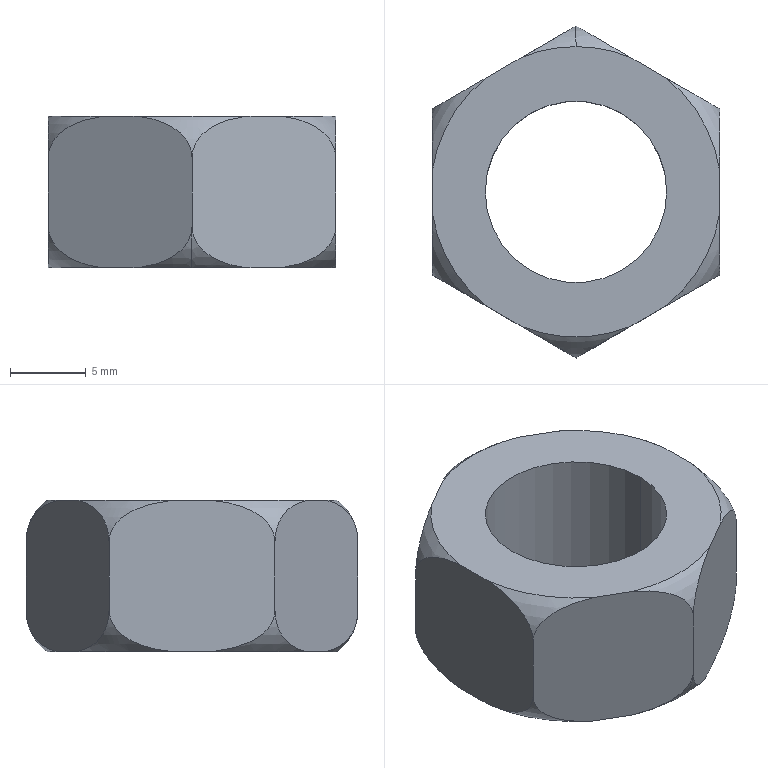Part | NX | 1 solid | 26 faces | box 19 x 21.939 x 10 mm | volume 1967 mm3 | torus 14 | plane 8 | cone 2 | cylinder 2 | commonest cylinder face diameters 12 x2
STEP:
#1=CARTESIAN_POINT('',(6.6,0.,-5.));
#2=VERTEX_POINT('',#1);
#3=CARTESIAN_POINT('',(-6.6,0.,-5.));
#4=VERTEX_POINT('',#3);
#5=CARTESIAN_POINT('',(0.,0.,-5.));
#6=DIRECTION('',(0.,0.,-1.));
#7=DIRECTION('',(-1.,0.,0.));
#8=AXIS2_PLACEMENT_3D('',#5,#6,#7);
#9=CIRCLE('',#8,6.6);
#10=EDGE_CURVE('',#2,#4,#9,.T.);
#11=ORIENTED_EDGE('',*,*,#10,.T.);
#12=CARTESIAN_POINT('',(-6.,0.,-4.4));
#13=VERTEX_POINT('',#12);
#14=CARTESIAN_POINT('',(-6.3,0.,-4.7));
#15=DIRECTION('',(-0.7071,0.,-0.7071));
#16=VECTOR('',#15,1000.);
#17=LINE('',#14,#16);
#18=EDGE_CURVE('',#4,#13,#17,.F.);
#19=ORIENTED_EDGE('',*,*,#18,.T.);
#20=CARTESIAN_POINT('',(6.,0.,-4.4));
#21=VERTEX_POINT('',#20);
#22=CARTESIAN_POINT('',(0.,0.,-4.4));
#23=DIRECTION('',(0.,0.,1.));
#24=DIRECTION('',(-1.,0.,0.));
#25=AXIS2_PLACEMENT_3D('',#22,#23,#24);
#26=CIRCLE('',#25,6.);
#27=EDGE_CURVE('',#13,#21,#26,.T.);
#28=ORIENTED_EDGE('',*,*,#27,.T.);
#29=CARTESIAN_POINT('',(6.3,0.,-4.7));
#30=DIRECTION('',(0.7071,0.,-0.7071));
#31=VECTOR('',#30,1000.);
#32=LINE('',#29,#31);
#33=EDGE_CURVE('',#2,#21,#32,.F.);
#34=ORIENTED_EDGE('',*,*,#33,.F.);
#35=EDGE_LOOP('',(#11,#19,#28,#34));
#36=FACE_BOUND('',#35,.T.);
#37=CARTESIAN_POINT('',(0.,0.,-4.7));
#38=DIRECTION('',(0.,0.,-1.));
#39=DIRECTION('',(-1.,0.,0.));
#40=AXIS2_PLACEMENT_3D('',#37,#38,#39);
#41=CONICAL_SURFACE('',#40,6.3,0.7854);
#42=ADVANCED_FACE('',(#36),#41,.F.);
#43=CARTESIAN_POINT('',(-6.,0.,5.));
#44=VERTEX_POINT('',#43);
#45=CARTESIAN_POINT('',(6.,0.,5.));
#46=VERTEX_POINT('',#45);
#47=CARTESIAN_POINT('',(0.,0.,5.));
#48=DIRECTION('',(0.,0.,1.));
#49=DIRECTION('',(-1.,0.,0.));
#50=AXIS2_PLACEMENT_3D('',#47,#48,#49);
#51=CIRCLE('',#50,6.);
#52=EDGE_CURVE('',#44,#46,#51,.T.);
#53=ORIENTED_EDGE('',*,*,#52,.T.);
#54=CARTESIAN_POINT('',(6.,0.,0.));
#55=DIRECTION('',(0.,0.,1.));
#56=VECTOR('',#55,1000.);
#57=LINE('',#54,#56);
#58=EDGE_CURVE('',#21,#46,#57,.T.);
#59=ORIENTED_EDGE('',*,*,#58,.F.);
#60=ORIENTED_EDGE('',*,*,#27,.F.);
#61=CARTESIAN_POINT('',(-6.,0.,0.));
#62=DIRECTION('',(0.,0.,1.));
#63=VECTOR('',#62,1000.);
#64=LINE('',#61,#63);
#65=EDGE_CURVE('',#13,#44,#64,.T.);
#66=ORIENTED_EDGE('',*,*,#65,.T.);
#67=EDGE_LOOP('',(#53,#59,#60,#66));
#68=FACE_BOUND('',#67,.T.);
#69=CARTESIAN_POINT('',(0.,0.,0.));
#70=DIRECTION('',(0.,0.,1.));
#71=DIRECTION('',(-1.,0.,0.));
#72=AXIS2_PLACEMENT_3D('',#69,#70,#71);
#73=CYLINDRICAL_SURFACE('',#72,6.);
#74=ADVANCED_FACE('',(#68),#73,.F.);
#75=CARTESIAN_POINT('',(5.938,7.542,-5.));
#76=VERTEX_POINT('',#75);
#77=CARTESIAN_POINT('',(9.5,1.371,-5.));
#78=VERTEX_POINT('',#77);
#79=CARTESIAN_POINT('',(0.,0.,-5.));
#80=DIRECTION('',(0.,0.,-1.));
#81=DIRECTION('',(-1.,0.,0.));
#82=AXIS2_PLACEMENT_3D('',#79,#80,#81);
#83=CIRCLE('',#82,9.598);
#84=EDGE_CURVE('',#76,#78,#83,.T.);
#85=ORIENTED_EDGE('',*,*,#84,.T.);
#86=CARTESIAN_POINT('',(9.5,-1.371,-5.));
#87=VERTEX_POINT('',#86);
#88=CARTESIAN_POINT('',(9.5,-1.371,-5.));
#89=DIRECTION('',(0.,1.,0.));
#90=VECTOR('',#89,1000.);
#91=LINE('',#88,#90);
#92=EDGE_CURVE('',#87,#78,#91,.T.);
#93=ORIENTED_EDGE('',*,*,#92,.F.);
#94=CARTESIAN_POINT('',(5.938,-7.542,-5.));
#95=VERTEX_POINT('',#94);
#96=CARTESIAN_POINT('',(0.,0.,-5.));
#97=DIRECTION('',(0.,0.,-1.));
#98=DIRECTION('',(-1.,0.,0.));
#99=AXIS2_PLACEMENT_3D('',#96,#97,#98);
#100=CIRCLE('',#99,9.598);
#101=EDGE_CURVE('',#87,#95,#100,.T.);
#102=ORIENTED_EDGE('',*,*,#101,.T.);
#103=CARTESIAN_POINT('',(3.562,-8.913,-5.));
#104=VERTEX_POINT('',#103);
#105=CARTESIAN_POINT('',(3.562,-8.913,-5.));
#106=DIRECTION('',(0.866,0.5,0.));
#107=VECTOR('',#106,1000.);
#108=LINE('',#105,#107);
#109=EDGE_CURVE('',#104,#95,#108,.T.);
#110=ORIENTED_EDGE('',*,*,#109,.F.);
#111=CARTESIAN_POINT('',(0.,-9.598,-5.));
#112=VERTEX_POINT('',#111);
#113=CARTESIAN_POINT('',(0.,0.,-5.));
#114=DIRECTION('',(0.,0.,-1.));
#115=DIRECTION('',(-1.,0.,0.));
#116=AXIS2_PLACEMENT_3D('',#113,#114,#115);
#117=CIRCLE('',#116,9.598);
#118=EDGE_CURVE('',#104,#112,#117,.T.);
#119=ORIENTED_EDGE('',*,*,#118,.T.);
#120=CARTESIAN_POINT('',(-3.562,-8.913,-5.));
#121=VERTEX_POINT('',#120);
#122=CARTESIAN_POINT('',(0.,0.,-5.));
#123=DIRECTION('',(0.,0.,-1.));
#124=DIRECTION('',(-1.,0.,0.));
#125=AXIS2_PLACEMENT_3D('',#122,#123,#124);
#126=CIRCLE('',#125,9.598);
#127=EDGE_CURVE('',#112,#121,#126,.T.);
#128=ORIENTED_EDGE('',*,*,#127,.T.);
#129=CARTESIAN_POINT('',(-5.938,-7.542,-5.));
#130=VERTEX_POINT('',#129);
#131=CARTESIAN_POINT('',(-5.938,-7.542,-5.));
#132=DIRECTION('',(0.866,-0.5,0.));
#133=VECTOR('',#132,1000.);
#134=LINE('',#131,#133);
#135=EDGE_CURVE('',#130,#121,#134,.T.);
#136=ORIENTED_EDGE('',*,*,#135,.F.);
#137=CARTESIAN_POINT('',(-9.5,-1.371,-5.));
#138=VERTEX_POINT('',#137);
#139=CARTESIAN_POINT('',(0.,0.,-5.));
#140=DIRECTION('',(0.,0.,-1.));
#141=DIRECTION('',(-1.,0.,0.));
#142=AXIS2_PLACEMENT_3D('',#139,#140,#141);
#143=CIRCLE('',#142,9.598);
#144=EDGE_CURVE('',#130,#138,#143,.T.);
#145=ORIENTED_EDGE('',*,*,#144,.T.);
#146=CARTESIAN_POINT('',(-9.5,1.371,-5.));
#147=VERTEX_POINT('',#146);
#148=CARTESIAN_POINT('',(-9.5,1.371,-5.));
#149=DIRECTION('',(0.,-1.,0.));
#150=VECTOR('',#149,1000.);
#151=LINE('',#148,#150);
#152=EDGE_CURVE('',#147,#138,#151,.T.);
#153=ORIENTED_EDGE('',*,*,#152,.F.);
#154=CARTESIAN_POINT('',(-5.938,7.542,-5.));
#155=VERTEX_POINT('',#154);
#156=CARTESIAN_POINT('',(0.,0.,-5.));
#157=DIRECTION('',(0.,0.,-1.));
#158=DIRECTION('',(-1.,0.,0.));
#159=AXIS2_PLACEMENT_3D('',#156,#157,#158);
#160=CIRCLE('',#159,9.598);
#161=EDGE_CURVE('',#147,#155,#160,.T.);
#162=ORIENTED_EDGE('',*,*,#161,.T.);
#163=CARTESIAN_POINT('',(-3.562,8.913,-5.));
#164=VERTEX_POINT('',#163);
#165=CARTESIAN_POINT('',(-3.562,8.913,-5.));
#166=DIRECTION('',(-0.866,-0.5,0.));
#167=VECTOR('',#166,1000.);
#168=LINE('',#165,#167);
#169=EDGE_CURVE('',#164,#155,#168,.T.);
#170=ORIENTED_EDGE('',*,*,#169,.F.);
#171=CARTESIAN_POINT('',(3.562,8.913,-5.));
#172=VERTEX_POINT('',#171);
#173=CARTESIAN_POINT('',(0.,0.,-5.));
#174=DIRECTION('',(0.,0.,-1.));
#175=DIRECTION('',(-1.,0.,0.));
#176=AXIS2_PLACEMENT_3D('',#173,#174,#175);
#177=CIRCLE('',#176,9.598);
#178=EDGE_CURVE('',#164,#172,#177,.T.);
#179=ORIENTED_EDGE('',*,*,#178,.T.);
#180=CARTESIAN_POINT('',(5.938,7.542,-5.));
#181=DIRECTION('',(-0.866,0.5,0.));
#182=VECTOR('',#181,1000.);
#183=LINE('',#180,#182);
#184=EDGE_CURVE('',#76,#172,#183,.T.);
#185=ORIENTED_EDGE('',*,*,#184,.F.);
#186=EDGE_LOOP('',(#85,#93,#102,#110,#119,#128,#136,#145,#153,#162,#170,#179,#185));
#187=FACE_BOUND('',#186,.T.);
#188=ORIENTED_EDGE('',*,*,#10,.F.);
#189=CARTESIAN_POINT('',(0.,0.,-5.));
#190=DIRECTION('',(0.,0.,-1.));
#191=DIRECTION('',(-1.,0.,0.));
#192=AXIS2_PLACEMENT_3D('',#189,#190,#191);
#193=CIRCLE('',#192,6.6);
#194=EDGE_CURVE('',#4,#2,#193,.T.);
#195=ORIENTED_EDGE('',*,*,#194,.F.);
#196=EDGE_LOOP('',(#188,#195));
#197=FACE_BOUND('',#196,.T.);
#198=CARTESIAN_POINT('',(0.,0.,-5.));
#199=DIRECTION('',(0.,0.,1.));
#200=DIRECTION('',(1.,0.,0.));
#201=AXIS2_PLACEMENT_3D('',#198,#199,#200);
#202=PLANE('',#201);
#203=ADVANCED_FACE('',(#187,#197),#202,.F.);
#204=CARTESIAN_POINT('',(-9.5,5.485,-2.258));
#205=VERTEX_POINT('',#204);
#206=CARTESIAN_POINT('',(-5.938,7.542,-5.));
#207=CARTESIAN_POINT('',(-6.359,7.298,-4.948));
#208=CARTESIAN_POINT('',(-6.904,6.984,-4.844));
#209=CARTESIAN_POINT('',(-7.693,6.528,-4.564));
#210=CARTESIAN_POINT('',(-8.328,6.161,-4.245));
#211=CARTESIAN_POINT('',(-9.176,5.672,-3.582));
#212=CARTESIAN_POINT('',(-9.5,5.485,-2.693));
#213=CARTESIAN_POINT('',(-9.5,5.485,-2.258));
#214=B_SPLINE_CURVE_WITH_KNOTS('',3,(#206,#207,#208,#209,#210,#211,#212,#213),.UNSPECIFIED.,.F.,.F.,(4,1,1,1,1,4),(0.,0.25,0.375,0.5,0.75,1.),.UNSPECIFIED.);
#215=EDGE_CURVE('',#155,#205,#214,.T.);
#216=ORIENTED_EDGE('',*,*,#215,.T.);
#217=CARTESIAN_POINT('',(-9.5,5.485,2.258));
#218=VERTEX_POINT('',#217);
#219=CARTESIAN_POINT('',(-9.5,5.485,2.258));
#220=DIRECTION('',(0.,0.,-1.));
#221=VECTOR('',#220,1000.);
#222=LINE('',#219,#221);
#223=EDGE_CURVE('',#218,#205,#222,.T.);
#224=ORIENTED_EDGE('',*,*,#223,.F.);
#225=CARTESIAN_POINT('',(-5.938,7.542,5.));
#226=VERTEX_POINT('',#225);
#227=CARTESIAN_POINT('',(-9.5,5.485,2.258));
#228=CARTESIAN_POINT('',(-9.5,5.485,2.477));
#229=CARTESIAN_POINT('',(-9.441,5.519,2.892));
#230=CARTESIAN_POINT('',(-9.089,5.722,3.534));
#231=CARTESIAN_POINT('',(-8.727,5.931,3.928));
#232=CARTESIAN_POINT('',(-8.146,6.266,4.343));
#233=CARTESIAN_POINT('',(-7.721,6.512,4.548));
#234=CARTESIAN_POINT('',(-7.,6.928,4.82));
#235=CARTESIAN_POINT('',(-6.388,7.281,4.944));
#236=CARTESIAN_POINT('',(-5.938,7.542,5.));
#237=B_SPLINE_CURVE_WITH_KNOTS('',3,(#227,#228,#229,#230,#231,#232,#233,#234,#235,#236),.UNSPECIFIED.,.F.,.F.,(4,1,1,1,1,1,1,4),(0.,0.125,0.25,0.375,0.5,0.625,0.75,1.),.UNSPECIFIED.);
#238=EDGE_CURVE('',#218,#226,#237,.T.);
#239=ORIENTED_EDGE('',*,*,#238,.T.);
#240=CARTESIAN_POINT('',(-3.562,8.913,5.));
#241=VERTEX_POINT('',#240);
#242=CARTESIAN_POINT('',(-5.938,7.542,5.));
#243=DIRECTION('',(0.866,0.5,0.));
#244=VECTOR('',#243,1000.);
#245=LINE('',#242,#244);
#246=EDGE_CURVE('',#226,#241,#245,.T.);
#247=ORIENTED_EDGE('',*,*,#246,.T.);
#248=CARTESIAN_POINT('',(0.,10.97,2.258));
#249=VERTEX_POINT('',#248);
#250=CARTESIAN_POINT('',(-3.562,8.913,5.));
#251=CARTESIAN_POINT('',(-3.141,9.156,4.948));
#252=CARTESIAN_POINT('',(-2.596,9.471,4.844));
#253=CARTESIAN_POINT('',(-1.807,9.926,4.564));
#254=CARTESIAN_POINT('',(-1.172,10.293,4.245));
#255=CARTESIAN_POINT('',(-0.3236,10.783,3.582));
#256=CARTESIAN_POINT('',(0.,10.97,2.693));
#257=CARTESIAN_POINT('',(0.,10.97,2.258));
#258=B_SPLINE_CURVE_WITH_KNOTS('',3,(#250,#251,#252,#253,#254,#255,#256,#257),.UNSPECIFIED.,.F.,.F.,(4,1,1,1,1,4),(0.,0.25,0.375,0.5,0.75,1.),.UNSPECIFIED.);
#259=EDGE_CURVE('',#241,#249,#258,.T.);
#260=ORIENTED_EDGE('',*,*,#259,.T.);
#261=CARTESIAN_POINT('',(0.,10.97,-2.258));
#262=VERTEX_POINT('',#261);
#263=CARTESIAN_POINT('',(0.,10.97,-2.258));
#264=DIRECTION('',(0.,0.,1.));
#265=VECTOR('',#264,1000.);
#266=LINE('',#263,#265);
#267=EDGE_CURVE('',#262,#249,#266,.T.);
#268=ORIENTED_EDGE('',*,*,#267,.F.);
#269=CARTESIAN_POINT('',(0.,10.97,-2.258));
#270=CARTESIAN_POINT('',(0.,10.97,-2.477));
#271=CARTESIAN_POINT('',(-0.05943,10.935,-2.892));
#272=CARTESIAN_POINT('',(-0.4107,10.733,-3.534));
#273=CARTESIAN_POINT('',(-0.7725,10.524,-3.928));
#274=CARTESIAN_POINT('',(-1.354,10.188,-4.343));
#275=CARTESIAN_POINT('',(-1.779,9.943,-4.548));
#276=CARTESIAN_POINT('',(-2.5,9.527,-4.82));
#277=CARTESIAN_POINT('',(-3.112,9.173,-4.944));
#278=CARTESIAN_POINT('',(-3.562,8.913,-5.));
#279=B_SPLINE_CURVE_WITH_KNOTS('',3,(#269,#270,#271,#272,#273,#274,#275,#276,#277,#278),.UNSPECIFIED.,.F.,.F.,(4,1,1,1,1,1,1,4),(0.,0.125,0.25,0.375,0.5,0.625,0.75,1.),.UNSPECIFIED.);
#280=EDGE_CURVE('',#262,#164,#279,.T.);
#281=ORIENTED_EDGE('',*,*,#280,.T.);
#282=ORIENTED_EDGE('',*,*,#169,.T.);
#283=EDGE_LOOP('',(#216,#224,#239,#247,#260,#268,#281,#282));
#284=FACE_BOUND('',#283,.T.);
#285=CARTESIAN_POINT('',(-9.5,5.485,0.));
#286=DIRECTION('',(-0.5,0.866,0.));
#287=DIRECTION('',(0.,0.,1.));
#288=AXIS2_PLACEMENT_3D('',#285,#286,#287);
#289=PLANE('',#288);
#290=ADVANCED_FACE('',(#284),#289,.T.);
#291=CARTESIAN_POINT('',(9.5,1.371,5.));
#292=VERTEX_POINT('',#291);
#293=CARTESIAN_POINT('',(5.938,7.542,5.));
#294=VERTEX_POINT('',#293);
#295=CARTESIAN_POINT('',(0.,0.,5.));
#296=DIRECTION('',(0.,0.,1.));
#297=DIRECTION('',(1.,0.,0.));
#298=AXIS2_PLACEMENT_3D('',#295,#296,#297);
#299=CIRCLE('',#298,9.598);
#300=EDGE_CURVE('',#292,#294,#299,.T.);
#301=ORIENTED_EDGE('',*,*,#300,.T.);
#302=CARTESIAN_POINT('',(3.562,8.913,5.));
#303=VERTEX_POINT('',#302);
#304=CARTESIAN_POINT('',(3.562,8.913,5.));
#305=DIRECTION('',(0.866,-0.5,0.));
#306=VECTOR('',#305,1000.);
#307=LINE('',#304,#306);
#308=EDGE_CURVE('',#303,#294,#307,.T.);
#309=ORIENTED_EDGE('',*,*,#308,.F.);
#310=CARTESIAN_POINT('',(0.,9.598,5.));
#311=VERTEX_POINT('',#310);
#312=CARTESIAN_POINT('',(0.,0.,5.));
#313=DIRECTION('',(0.,0.,1.));
#314=DIRECTION('',(1.,0.,0.));
#315=AXIS2_PLACEMENT_3D('',#312,#313,#314);
#316=CIRCLE('',#315,9.598);
#317=EDGE_CURVE('',#303,#311,#316,.T.);
#318=ORIENTED_EDGE('',*,*,#317,.T.);
#319=CARTESIAN_POINT('',(0.,0.,5.));
#320=DIRECTION('',(0.,0.,1.));
#321=DIRECTION('',(1.,0.,0.));
#322=AXIS2_PLACEMENT_3D('',#319,#320,#321);
#323=CIRCLE('',#322,9.598);
#324=EDGE_CURVE('',#311,#241,#323,.T.);
#325=ORIENTED_EDGE('',*,*,#324,.T.);
#326=ORIENTED_EDGE('',*,*,#246,.F.);
#327=CARTESIAN_POINT('',(-9.5,1.371,5.));
#328=VERTEX_POINT('',#327);
#329=CARTESIAN_POINT('',(0.,0.,5.));
#330=DIRECTION('',(0.,0.,1.));
#331=DIRECTION('',(1.,0.,0.));
#332=AXIS2_PLACEMENT_3D('',#329,#330,#331);
#333=CIRCLE('',#332,9.598);
#334=EDGE_CURVE('',#226,#328,#333,.T.);
#335=ORIENTED_EDGE('',*,*,#334,.T.);
#336=CARTESIAN_POINT('',(-9.5,-1.371,5.));
#337=VERTEX_POINT('',#336);
#338=CARTESIAN_POINT('',(-9.5,-1.371,5.));
#339=DIRECTION('',(0.,1.,0.));
#340=VECTOR('',#339,1000.);
#341=LINE('',#338,#340);
#342=EDGE_CURVE('',#337,#328,#341,.T.);
#343=ORIENTED_EDGE('',*,*,#342,.F.);
#344=CARTESIAN_POINT('',(-5.938,-7.542,5.));
#345=VERTEX_POINT('',#344);
#346=CARTESIAN_POINT('',(0.,0.,5.));
#347=DIRECTION('',(0.,0.,1.));
#348=DIRECTION('',(1.,0.,0.));
#349=AXIS2_PLACEMENT_3D('',#346,#347,#348);
#350=CIRCLE('',#349,9.598);
#351=EDGE_CURVE('',#337,#345,#350,.T.);
#352=ORIENTED_EDGE('',*,*,#351,.T.);
#353=CARTESIAN_POINT('',(-3.562,-8.913,5.));
#354=VERTEX_POINT('',#353);
#355=CARTESIAN_POINT('',(-3.562,-8.913,5.));
#356=DIRECTION('',(-0.866,0.5,0.));
#357=VECTOR('',#356,1000.);
#358=LINE('',#355,#357);
#359=EDGE_CURVE('',#354,#345,#358,.T.);
#360=ORIENTED_EDGE('',*,*,#359,.F.);
#361=CARTESIAN_POINT('',(3.562,-8.913,5.));
#362=VERTEX_POINT('',#361);
#363=CARTESIAN_POINT('',(0.,0.,5.));
#364=DIRECTION('',(0.,0.,1.));
#365=DIRECTION('',(1.,0.,0.));
#366=AXIS2_PLACEMENT_3D('',#363,#364,#365);
#367=CIRCLE('',#366,9.598);
#368=EDGE_CURVE('',#354,#362,#367,.T.);
#369=ORIENTED_EDGE('',*,*,#368,.T.);
#370=CARTESIAN_POINT('',(5.938,-7.542,5.));
#371=VERTEX_POINT('',#370);
#372=CARTESIAN_POINT('',(5.938,-7.542,5.));
#373=DIRECTION('',(-0.866,-0.5,0.));
#374=VECTOR('',#373,1000.);
#375=LINE('',#372,#374);
#376=EDGE_CURVE('',#371,#362,#375,.T.);
#377=ORIENTED_EDGE('',*,*,#376,.F.);
#378=CARTESIAN_POINT('',(9.5,-1.371,5.));
#379=VERTEX_POINT('',#378);
#380=CARTESIAN_POINT('',(0.,0.,5.));
#381=DIRECTION('',(0.,0.,1.));
#382=DIRECTION('',(1.,0.,0.));
#383=AXIS2_PLACEMENT_3D('',#380,#381,#382);
#384=CIRCLE('',#383,9.598);
#385=EDGE_CURVE('',#371,#379,#384,.T.);
#386=ORIENTED_EDGE('',*,*,#385,.T.);
#387=CARTESIAN_POINT('',(9.5,1.371,5.));
#388=DIRECTION('',(0.,-1.,0.));
#389=VECTOR('',#388,1000.);
#390=LINE('',#387,#389);
#391=EDGE_CURVE('',#292,#379,#390,.T.);
#392=ORIENTED_EDGE('',*,*,#391,.F.);
#393=EDGE_LOOP('',(#301,#309,#318,#325,#326,#335,#343,#352,#360,#369,#377,#386,#392));
#394=FACE_BOUND('',#393,.T.);
#395=ORIENTED_EDGE('',*,*,#52,.F.);
#396=CARTESIAN_POINT('',(0.,0.,5.));
#397=DIRECTION('',(0.,0.,1.));
#398=DIRECTION('',(-1.,0.,0.));
#399=AXIS2_PLACEMENT_3D('',#396,#397,#398);
#400=CIRCLE('',#399,6.);
#401=EDGE_CURVE('',#46,#44,#400,.T.);
#402=ORIENTED_EDGE('',*,*,#401,.F.);
#403=EDGE_LOOP('',(#395,#402));
#404=FACE_BOUND('',#403,.T.);
#405=CARTESIAN_POINT('',(0.,0.,5.));
#406=DIRECTION('',(0.,0.,1.));
#407=DIRECTION('',(1.,0.,0.));
#408=AXIS2_PLACEMENT_3D('',#405,#406,#407);
#409=PLANE('',#408);
#410=ADVANCED_FACE('',(#394,#404),#409,.T.);
#411=ORIENTED_EDGE('',*,*,#215,.F.);
#412=ORIENTED_EDGE('',*,*,#161,.F.);
#413=CARTESIAN_POINT('',(-9.5,5.485,-2.258));
#414=CARTESIAN_POINT('',(-9.5,5.485,-2.477));
#415=CARTESIAN_POINT('',(-9.5,5.416,-2.892));
#416=CARTESIAN_POINT('',(-9.5,5.011,-3.534));
#417=CARTESIAN_POINT('',(-9.5,4.593,-3.928));
#418=CARTESIAN_POINT('',(-9.5,3.922,-4.343));
#419=CARTESIAN_POINT('',(-9.5,3.431,-4.548));
#420=CARTESIAN_POINT('',(-9.5,2.599,-4.82));
#421=CARTESIAN_POINT('',(-9.5,1.892,-4.944));
#422=CARTESIAN_POINT('',(-9.5,1.371,-5.));
#423=B_SPLINE_CURVE_WITH_KNOTS('',3,(#413,#414,#415,#416,#417,#418,#419,#420,#421,#422),.UNSPECIFIED.,.F.,.F.,(4,1,1,1,1,1,1,4),(0.,0.125,0.25,0.375,0.5,0.625,0.75,1.),.UNSPECIFIED.);
#424=EDGE_CURVE('',#205,#147,#423,.T.);
#425=ORIENTED_EDGE('',*,*,#424,.F.);
#426=EDGE_LOOP('',(#411,#412,#425));
#427=FACE_BOUND('',#426,.T.);
#428=CARTESIAN_POINT('',(0.,0.,-2.258));
#429=DIRECTION('',(0.,0.,1.));
#430=DIRECTION('',(0.,1.,0.));
#431=AXIS2_PLACEMENT_3D('',#428,#429,#430);
#432=TOROIDAL_SURFACE('',#431,7.542,3.428);
#433=ADVANCED_FACE('',(#427),#432,.T.);
#434=CARTESIAN_POINT('',(-9.5,-5.485,-2.258));
#435=VERTEX_POINT('',#434);
#436=CARTESIAN_POINT('',(-9.5,-1.371,-5.));
#437=CARTESIAN_POINT('',(-9.5,-1.858,-4.948));
#438=CARTESIAN_POINT('',(-9.5,-2.487,-4.844));
#439=CARTESIAN_POINT('',(-9.5,-3.398,-4.564));
#440=CARTESIAN_POINT('',(-9.5,-4.132,-4.245));
#441=CARTESIAN_POINT('',(-9.5,-5.111,-3.582));
#442=CARTESIAN_POINT('',(-9.5,-5.485,-2.693));
#443=CARTESIAN_POINT('',(-9.5,-5.485,-2.258));
#444=B_SPLINE_CURVE_WITH_KNOTS('',3,(#436,#437,#438,#439,#440,#441,#442,#443),.UNSPECIFIED.,.F.,.F.,(4,1,1,1,1,4),(0.,0.25,0.375,0.5,0.75,1.),.UNSPECIFIED.);
#445=EDGE_CURVE('',#138,#435,#444,.T.);
#446=ORIENTED_EDGE('',*,*,#445,.F.);
#447=ORIENTED_EDGE('',*,*,#144,.F.);
#448=CARTESIAN_POINT('',(-9.5,-5.485,-2.258));
#449=CARTESIAN_POINT('',(-9.5,-5.485,-2.477));
#450=CARTESIAN_POINT('',(-9.441,-5.519,-2.892));
#451=CARTESIAN_POINT('',(-9.089,-5.722,-3.534));
#452=CARTESIAN_POINT('',(-8.727,-5.931,-3.928));
#453=CARTESIAN_POINT('',(-8.146,-6.266,-4.343));
#454=CARTESIAN_POINT('',(-7.721,-6.512,-4.548));
#455=CARTESIAN_POINT('',(-7.,-6.928,-4.82));
#456=CARTESIAN_POINT('',(-6.388,-7.281,-4.944));
#457=CARTESIAN_POINT('',(-5.938,-7.542,-5.));
#458=B_SPLINE_CURVE_WITH_KNOTS('',3,(#448,#449,#450,#451,#452,#453,#454,#455,#456,#457),.UNSPECIFIED.,.F.,.F.,(4,1,1,1,1,1,1,4),(0.,0.125,0.25,0.375,0.5,0.625,0.75,1.),.UNSPECIFIED.);
#459=EDGE_CURVE('',#435,#130,#458,.T.);
#460=ORIENTED_EDGE('',*,*,#459,.F.);
#461=EDGE_LOOP('',(#446,#447,#460));
#462=FACE_BOUND('',#461,.T.);
#463=CARTESIAN_POINT('',(0.,0.,-2.258));
#464=DIRECTION('',(0.,0.,1.));
#465=DIRECTION('',(0.,1.,0.));
#466=AXIS2_PLACEMENT_3D('',#463,#464,#465);
#467=TOROIDAL_SURFACE('',#466,7.542,3.428);
#468=ADVANCED_FACE('',(#462),#467,.T.);
#469=CARTESIAN_POINT('',(0.,-10.97,-2.258));
#470=VERTEX_POINT('',#469);
#471=CARTESIAN_POINT('',(0.,-7.542,-2.258));
#472=DIRECTION('',(1.,0.,0.));
#473=DIRECTION('',(0.,0.,-1.));
#474=AXIS2_PLACEMENT_3D('',#471,#472,#473);
#475=CIRCLE('',#474,3.428);
#476=EDGE_CURVE('',#470,#112,#475,.T.);
#477=ORIENTED_EDGE('',*,*,#476,.F.);
#478=CARTESIAN_POINT('',(-3.562,-8.913,-5.));
#479=CARTESIAN_POINT('',(-3.141,-9.156,-4.948));
#480=CARTESIAN_POINT('',(-2.596,-9.471,-4.844));
#481=CARTESIAN_POINT('',(-1.807,-9.926,-4.564));
#482=CARTESIAN_POINT('',(-1.172,-10.293,-4.245));
#483=CARTESIAN_POINT('',(-0.3236,-10.783,-3.582));
#484=CARTESIAN_POINT('',(0.,-10.97,-2.693));
#485=CARTESIAN_POINT('',(0.,-10.97,-2.258));
#486=B_SPLINE_CURVE_WITH_KNOTS('',3,(#478,#479,#480,#481,#482,#483,#484,#485),.UNSPECIFIED.,.F.,.F.,(4,1,1,1,1,4),(0.,0.25,0.375,0.5,0.75,1.),.UNSPECIFIED.);
#487=EDGE_CURVE('',#121,#470,#486,.T.);
#488=ORIENTED_EDGE('',*,*,#487,.F.);
#489=ORIENTED_EDGE('',*,*,#127,.F.);
#490=EDGE_LOOP('',(#477,#488,#489));
#491=FACE_BOUND('',#490,.T.);
#492=CARTESIAN_POINT('',(0.,0.,-2.258));
#493=DIRECTION('',(0.,0.,-1.));
#494=DIRECTION('',(0.,-1.,0.));
#495=AXIS2_PLACEMENT_3D('',#492,#493,#494);
#496=TOROIDAL_SURFACE('',#495,7.542,3.428);
#497=ADVANCED_FACE('',(#491),#496,.T.);
#498=CARTESIAN_POINT('',(3.562,8.913,-5.));
#499=CARTESIAN_POINT('',(3.141,9.156,-4.948));
#500=CARTESIAN_POINT('',(2.596,9.471,-4.844));
#501=CARTESIAN_POINT('',(1.807,9.926,-4.564));
#502=CARTESIAN_POINT('',(1.172,10.293,-4.245));
#503=CARTESIAN_POINT('',(0.3236,10.783,-3.582));
#504=CARTESIAN_POINT('',(0.,10.97,-2.693));
#505=CARTESIAN_POINT('',(0.,10.97,-2.258));
#506=B_SPLINE_CURVE_WITH_KNOTS('',3,(#498,#499,#500,#501,#502,#503,#504,#505),.UNSPECIFIED.,.F.,.F.,(4,1,1,1,1,4),(0.,0.25,0.375,0.5,0.75,1.),.UNSPECIFIED.);
#507=EDGE_CURVE('',#172,#262,#506,.T.);
#508=ORIENTED_EDGE('',*,*,#507,.F.);
#509=ORIENTED_EDGE('',*,*,#178,.F.);
#510=ORIENTED_EDGE('',*,*,#280,.F.);
#511=EDGE_LOOP('',(#508,#509,#510));
#512=FACE_BOUND('',#511,.T.);
#513=CARTESIAN_POINT('',(0.,0.,-2.258));
#514=DIRECTION('',(0.,0.,-1.));
#515=DIRECTION('',(0.,-1.,0.));
#516=AXIS2_PLACEMENT_3D('',#513,#514,#515);
#517=TOROIDAL_SURFACE('',#516,7.542,3.428);
#518=ADVANCED_FACE('',(#512),#517,.T.);
#519=CARTESIAN_POINT('',(9.5,-5.485,-2.258));
#520=VERTEX_POINT('',#519);
#521=CARTESIAN_POINT('',(5.938,-7.542,-5.));
#522=CARTESIAN_POINT('',(6.359,-7.298,-4.948));
#523=CARTESIAN_POINT('',(6.904,-6.984,-4.844));
#524=CARTESIAN_POINT('',(7.693,-6.528,-4.564));
#525=CARTESIAN_POINT('',(8.328,-6.161,-4.245));
#526=CARTESIAN_POINT('',(9.176,-5.672,-3.582));
#527=CARTESIAN_POINT('',(9.5,-5.485,-2.693));
#528=CARTESIAN_POINT('',(9.5,-5.485,-2.258));
#529=B_SPLINE_CURVE_WITH_KNOTS('',3,(#521,#522,#523,#524,#525,#526,#527,#528),.UNSPECIFIED.,.F.,.F.,(4,1,1,1,1,4),(0.,0.25,0.375,0.5,0.75,1.),.UNSPECIFIED.);
#530=EDGE_CURVE('',#95,#520,#529,.T.);
#531=ORIENTED_EDGE('',*,*,#530,.F.);
#532=ORIENTED_EDGE('',*,*,#101,.F.);
#533=CARTESIAN_POINT('',(9.5,-5.485,-2.258));
#534=CARTESIAN_POINT('',(9.5,-5.485,-2.477));
#535=CARTESIAN_POINT('',(9.5,-5.416,-2.892));
#536=CARTESIAN_POINT('',(9.5,-5.011,-3.534));
#537=CARTESIAN_POINT('',(9.5,-4.593,-3.928));
#538=CARTESIAN_POINT('',(9.5,-3.922,-4.343));
#539=CARTESIAN_POINT('',(9.5,-3.431,-4.548));
#540=CARTESIAN_POINT('',(9.5,-2.599,-4.82));
#541=CARTESIAN_POINT('',(9.5,-1.892,-4.944));
#542=CARTESIAN_POINT('',(9.5,-1.371,-5.));
#543=B_SPLINE_CURVE_WITH_KNOTS('',3,(#533,#534,#535,#536,#537,#538,#539,#540,#541,#542),.UNSPECIFIED.,.F.,.F.,(4,1,1,1,1,1,1,4),(0.,0.125,0.25,0.375,0.5,0.625,0.75,1.),.UNSPECIFIED.);
#544=EDGE_CURVE('',#520,#87,#543,.T.);
#545=ORIENTED_EDGE('',*,*,#544,.F.);
#546=EDGE_LOOP('',(#531,#532,#545));
#547=FACE_BOUND('',#546,.T.);
#548=CARTESIAN_POINT('',(0.,0.,-2.258));
#549=DIRECTION('',(0.,0.,1.));
#550=DIRECTION('',(0.,1.,0.));
#551=AXIS2_PLACEMENT_3D('',#548,#549,#550);
#552=TOROIDAL_SURFACE('',#551,7.542,3.428);
#553=ADVANCED_FACE('',(#547),#552,.T.);
#554=CARTESIAN_POINT('',(9.5,5.485,-2.258));
#555=VERTEX_POINT('',#554);
#556=CARTESIAN_POINT('',(9.5,1.371,-5.));
#557=CARTESIAN_POINT('',(9.5,1.858,-4.948));
#558=CARTESIAN_POINT('',(9.5,2.487,-4.844));
#559=CARTESIAN_POINT('',(9.5,3.398,-4.564));
#560=CARTESIAN_POINT('',(9.5,4.132,-4.245));
#561=CARTESIAN_POINT('',(9.5,5.111,-3.582));
#562=CARTESIAN_POINT('',(9.5,5.485,-2.693));
#563=CARTESIAN_POINT('',(9.5,5.485,-2.258));
#564=B_SPLINE_CURVE_WITH_KNOTS('',3,(#556,#557,#558,#559,#560,#561,#562,#563),.UNSPECIFIED.,.F.,.F.,(4,1,1,1,1,4),(0.,0.25,0.375,0.5,0.75,1.),.UNSPECIFIED.);
#565=EDGE_CURVE('',#78,#555,#564,.T.);
#566=ORIENTED_EDGE('',*,*,#565,.F.);
#567=ORIENTED_EDGE('',*,*,#84,.F.);
#568=CARTESIAN_POINT('',(9.5,5.485,-2.258));
#569=CARTESIAN_POINT('',(9.5,5.485,-2.477));
#570=CARTESIAN_POINT('',(9.441,5.519,-2.892));
#571=CARTESIAN_POINT('',(9.089,5.722,-3.534));
#572=CARTESIAN_POINT('',(8.727,5.931,-3.928));
#573=CARTESIAN_POINT('',(8.146,6.266,-4.343));
#574=CARTESIAN_POINT('',(7.721,6.512,-4.548));
#575=CARTESIAN_POINT('',(7.,6.928,-4.82));
#576=CARTESIAN_POINT('',(6.388,7.281,-4.944));
#577=CARTESIAN_POINT('',(5.938,7.542,-5.));
#578=B_SPLINE_CURVE_WITH_KNOTS('',3,(#568,#569,#570,#571,#572,#573,#574,#575,#576,#577),.UNSPECIFIED.,.F.,.F.,(4,1,1,1,1,1,1,4),(0.,0.125,0.25,0.375,0.5,0.625,0.75,1.),.UNSPECIFIED.);
#579=EDGE_CURVE('',#555,#76,#578,.T.);
#580=ORIENTED_EDGE('',*,*,#579,.F.);
#581=EDGE_LOOP('',(#566,#567,#580));
#582=FACE_BOUND('',#581,.T.);
#583=CARTESIAN_POINT('',(0.,0.,-2.258));
#584=DIRECTION('',(0.,0.,1.));
#585=DIRECTION('',(0.,1.,0.));
#586=AXIS2_PLACEMENT_3D('',#583,#584,#585);
#587=TOROIDAL_SURFACE('',#586,7.542,3.428);
#588=ADVANCED_FACE('',(#582),#587,.T.);
#589=ORIENTED_EDGE('',*,*,#565,.T.);
#590=CARTESIAN_POINT('',(9.5,5.485,2.258));
#591=VERTEX_POINT('',#590);
#592=CARTESIAN_POINT('',(9.5,5.485,2.258));
#593=DIRECTION('',(0.,0.,-1.));
#594=VECTOR('',#593,1000.);
#595=LINE('',#592,#594);
#596=EDGE_CURVE('',#591,#555,#595,.T.);
#597=ORIENTED_EDGE('',*,*,#596,.F.);
#598=CARTESIAN_POINT('',(9.5,5.485,2.258));
#599=CARTESIAN_POINT('',(9.5,5.485,2.477));
#600=CARTESIAN_POINT('',(9.5,5.416,2.892));
#601=CARTESIAN_POINT('',(9.5,5.011,3.534));
#602=CARTESIAN_POINT('',(9.5,4.593,3.928));
#603=CARTESIAN_POINT('',(9.5,3.922,4.343));
#604=CARTESIAN_POINT('',(9.5,3.431,4.548));
#605=CARTESIAN_POINT('',(9.5,2.599,4.82));
#606=CARTESIAN_POINT('',(9.5,1.892,4.944));
#607=CARTESIAN_POINT('',(9.5,1.371,5.));
#608=B_SPLINE_CURVE_WITH_KNOTS('',3,(#598,#599,#600,#601,#602,#603,#604,#605,#606,#607),.UNSPECIFIED.,.F.,.F.,(4,1,1,1,1,1,1,4),(0.,0.125,0.25,0.375,0.5,0.625,0.75,1.),.UNSPECIFIED.);
#609=EDGE_CURVE('',#591,#292,#608,.T.);
#610=ORIENTED_EDGE('',*,*,#609,.T.);
#611=ORIENTED_EDGE('',*,*,#391,.T.);
#612=CARTESIAN_POINT('',(9.5,-5.485,2.258));
#613=VERTEX_POINT('',#612);
#614=CARTESIAN_POINT('',(9.5,-1.371,5.));
#615=CARTESIAN_POINT('',(9.5,-1.858,4.948));
#616=CARTESIAN_POINT('',(9.5,-2.487,4.844));
#617=CARTESIAN_POINT('',(9.5,-3.398,4.564));
#618=CARTESIAN_POINT('',(9.5,-4.132,4.245));
#619=CARTESIAN_POINT('',(9.5,-5.111,3.582));
#620=CARTESIAN_POINT('',(9.5,-5.485,2.693));
#621=CARTESIAN_POINT('',(9.5,-5.485,2.258));
#622=B_SPLINE_CURVE_WITH_KNOTS('',3,(#614,#615,#616,#617,#618,#619,#620,#621),.UNSPECIFIED.,.F.,.F.,(4,1,1,1,1,4),(0.,0.25,0.375,0.5,0.75,1.),.UNSPECIFIED.);
#623=EDGE_CURVE('',#379,#613,#622,.T.);
#624=ORIENTED_EDGE('',*,*,#623,.T.);
#625=CARTESIAN_POINT('',(9.5,-5.485,2.258));
#626=DIRECTION('',(0.,0.,-1.));
#627=VECTOR('',#626,1000.);
#628=LINE('',#625,#627);
#629=EDGE_CURVE('',#613,#520,#628,.T.);
#630=ORIENTED_EDGE('',*,*,#629,.T.);
#631=ORIENTED_EDGE('',*,*,#544,.T.);
#632=ORIENTED_EDGE('',*,*,#92,.T.);
#633=EDGE_LOOP('',(#589,#597,#610,#611,#624,#630,#631,#632));
#634=FACE_BOUND('',#633,.T.);
#635=CARTESIAN_POINT('',(9.5,5.485,0.));
#636=DIRECTION('',(1.,0.,0.));
#637=DIRECTION('',(0.,1.,0.));
#638=AXIS2_PLACEMENT_3D('',#635,#636,#637);
#639=PLANE('',#638);
#640=ADVANCED_FACE('',(#634),#639,.T.);
#641=ORIENTED_EDGE('',*,*,#238,.F.);
#642=CARTESIAN_POINT('',(-9.5,1.371,5.));
#643=CARTESIAN_POINT('',(-9.5,1.858,4.948));
#644=CARTESIAN_POINT('',(-9.5,2.487,4.844));
#645=CARTESIAN_POINT('',(-9.5,3.398,4.564));
#646=CARTESIAN_POINT('',(-9.5,4.132,4.245));
#647=CARTESIAN_POINT('',(-9.5,5.111,3.582));
#648=CARTESIAN_POINT('',(-9.5,5.485,2.693));
#649=CARTESIAN_POINT('',(-9.5,5.485,2.258));
#650=B_SPLINE_CURVE_WITH_KNOTS('',3,(#642,#643,#644,#645,#646,#647,#648,#649),.UNSPECIFIED.,.F.,.F.,(4,1,1,1,1,4),(0.,0.25,0.375,0.5,0.75,1.),.UNSPECIFIED.);
#651=EDGE_CURVE('',#328,#218,#650,.T.);
#652=ORIENTED_EDGE('',*,*,#651,.F.);
#653=ORIENTED_EDGE('',*,*,#334,.F.);
#654=EDGE_LOOP('',(#641,#652,#653));
#655=FACE_BOUND('',#654,.T.);
#656=CARTESIAN_POINT('',(0.,0.,2.258));
#657=DIRECTION('',(0.,0.,-1.));
#658=DIRECTION('',(0.,-1.,0.));
#659=AXIS2_PLACEMENT_3D('',#656,#657,#658);
#660=TOROIDAL_SURFACE('',#659,7.542,3.428);
#661=ADVANCED_FACE('',(#655),#660,.T.);
#662=CARTESIAN_POINT('',(-9.5,-5.485,2.258));
#663=VERTEX_POINT('',#662);
#664=CARTESIAN_POINT('',(-9.5,-5.485,2.258));
#665=CARTESIAN_POINT('',(-9.5,-5.485,2.477));
#666=CARTESIAN_POINT('',(-9.5,-5.416,2.892));
#667=CARTESIAN_POINT('',(-9.5,-5.011,3.534));
#668=CARTESIAN_POINT('',(-9.5,-4.593,3.928));
#669=CARTESIAN_POINT('',(-9.5,-3.922,4.343));
#670=CARTESIAN_POINT('',(-9.5,-3.431,4.548));
#671=CARTESIAN_POINT('',(-9.5,-2.599,4.82));
#672=CARTESIAN_POINT('',(-9.5,-1.892,4.944));
#673=CARTESIAN_POINT('',(-9.5,-1.371,5.));
#674=B_SPLINE_CURVE_WITH_KNOTS('',3,(#664,#665,#666,#667,#668,#669,#670,#671,#672,#673),.UNSPECIFIED.,.F.,.F.,(4,1,1,1,1,1,1,4),(0.,0.125,0.25,0.375,0.5,0.625,0.75,1.),.UNSPECIFIED.);
#675=EDGE_CURVE('',#663,#337,#674,.T.);
#676=ORIENTED_EDGE('',*,*,#675,.F.);
#677=CARTESIAN_POINT('',(-5.938,-7.542,5.));
#678=CARTESIAN_POINT('',(-6.359,-7.298,4.948));
#679=CARTESIAN_POINT('',(-6.904,-6.984,4.844));
#680=CARTESIAN_POINT('',(-7.693,-6.528,4.564));
#681=CARTESIAN_POINT('',(-8.328,-6.161,4.245));
#682=CARTESIAN_POINT('',(-9.176,-5.672,3.582));
#683=CARTESIAN_POINT('',(-9.5,-5.485,2.693));
#684=CARTESIAN_POINT('',(-9.5,-5.485,2.258));
#685=B_SPLINE_CURVE_WITH_KNOTS('',3,(#677,#678,#679,#680,#681,#682,#683,#684),.UNSPECIFIED.,.F.,.F.,(4,1,1,1,1,4),(0.,0.25,0.375,0.5,0.75,1.),.UNSPECIFIED.);
#686=EDGE_CURVE('',#345,#663,#685,.T.);
#687=ORIENTED_EDGE('',*,*,#686,.F.);
#688=ORIENTED_EDGE('',*,*,#351,.F.);
#689=EDGE_LOOP('',(#676,#687,#688));
#690=FACE_BOUND('',#689,.T.);
#691=CARTESIAN_POINT('',(0.,0.,2.258));
#692=DIRECTION('',(0.,0.,-1.));
#693=DIRECTION('',(0.,-1.,0.));
#694=AXIS2_PLACEMENT_3D('',#691,#692,#693);
#695=TOROIDAL_SURFACE('',#694,7.542,3.428);
#696=ADVANCED_FACE('',(#690),#695,.T.);
#697=CARTESIAN_POINT('',(0.,-10.97,2.258));
#698=VERTEX_POINT('',#697);
#699=CARTESIAN_POINT('',(0.,-10.97,2.258));
#700=CARTESIAN_POINT('',(0.,-10.97,2.477));
#701=CARTESIAN_POINT('',(-0.05943,-10.935,2.892));
#702=CARTESIAN_POINT('',(-0.4107,-10.733,3.534));
#703=CARTESIAN_POINT('',(-0.7725,-10.524,3.928));
#704=CARTESIAN_POINT('',(-1.354,-10.188,4.343));
#705=CARTESIAN_POINT('',(-1.779,-9.943,4.548));
#706=CARTESIAN_POINT('',(-2.5,-9.527,4.82));
#707=CARTESIAN_POINT('',(-3.112,-9.173,4.944));
#708=CARTESIAN_POINT('',(-3.562,-8.913,5.));
#709=B_SPLINE_CURVE_WITH_KNOTS('',3,(#699,#700,#701,#702,#703,#704,#705,#706,#707,#708),.UNSPECIFIED.,.F.,.F.,(4,1,1,1,1,1,1,4),(0.,0.125,0.25,0.375,0.5,0.625,0.75,1.),.UNSPECIFIED.);
#710=EDGE_CURVE('',#698,#354,#709,.T.);
#711=ORIENTED_EDGE('',*,*,#710,.F.);
#712=CARTESIAN_POINT('',(3.562,-8.913,5.));
#713=CARTESIAN_POINT('',(3.141,-9.156,4.948));
#714=CARTESIAN_POINT('',(2.596,-9.471,4.844));
#715=CARTESIAN_POINT('',(1.807,-9.926,4.564));
#716=CARTESIAN_POINT('',(1.172,-10.293,4.245));
#717=CARTESIAN_POINT('',(0.3236,-10.783,3.582));
#718=CARTESIAN_POINT('',(0.,-10.97,2.693));
#719=CARTESIAN_POINT('',(0.,-10.97,2.258));
#720=B_SPLINE_CURVE_WITH_KNOTS('',3,(#712,#713,#714,#715,#716,#717,#718,#719),.UNSPECIFIED.,.F.,.F.,(4,1,1,1,1,4),(0.,0.25,0.375,0.5,0.75,1.),.UNSPECIFIED.);
#721=EDGE_CURVE('',#362,#698,#720,.T.);
#722=ORIENTED_EDGE('',*,*,#721,.F.);
#723=ORIENTED_EDGE('',*,*,#368,.F.);
#724=EDGE_LOOP('',(#711,#722,#723));
#725=FACE_BOUND('',#724,.T.);
#726=CARTESIAN_POINT('',(0.,0.,2.258));
#727=DIRECTION('',(0.,0.,1.));
#728=DIRECTION('',(0.,1.,0.));
#729=AXIS2_PLACEMENT_3D('',#726,#727,#728);
#730=TOROIDAL_SURFACE('',#729,7.542,3.428);
#731=ADVANCED_FACE('',(#725),#730,.T.);
#732=CARTESIAN_POINT('',(9.5,-5.485,2.258));
#733=CARTESIAN_POINT('',(9.5,-5.485,2.477));
#734=CARTESIAN_POINT('',(9.441,-5.519,2.892));
#735=CARTESIAN_POINT('',(9.089,-5.722,3.534));
#736=CARTESIAN_POINT('',(8.727,-5.931,3.928));
#737=CARTESIAN_POINT('',(8.146,-6.266,4.343));
#738=CARTESIAN_POINT('',(7.721,-6.512,4.548));
#739=CARTESIAN_POINT('',(7.,-6.928,4.82));
#740=CARTESIAN_POINT('',(6.388,-7.281,4.944));
#741=CARTESIAN_POINT('',(5.938,-7.542,5.));
#742=B_SPLINE_CURVE_WITH_KNOTS('',3,(#732,#733,#734,#735,#736,#737,#738,#739,#740,#741),.UNSPECIFIED.,.F.,.F.,(4,1,1,1,1,1,1,4),(0.,0.125,0.25,0.375,0.5,0.625,0.75,1.),.UNSPECIFIED.);
#743=EDGE_CURVE('',#613,#371,#742,.T.);
#744=ORIENTED_EDGE('',*,*,#743,.F.);
#745=ORIENTED_EDGE('',*,*,#623,.F.);
#746=ORIENTED_EDGE('',*,*,#385,.F.);
#747=EDGE_LOOP('',(#744,#745,#746));
#748=FACE_BOUND('',#747,.T.);
#749=CARTESIAN_POINT('',(0.,0.,2.258));
#750=DIRECTION('',(0.,0.,-1.));
#751=DIRECTION('',(0.,-1.,0.));
#752=AXIS2_PLACEMENT_3D('',#749,#750,#751);
#753=TOROIDAL_SURFACE('',#752,7.542,3.428);
#754=ADVANCED_FACE('',(#748),#753,.T.);
#755=CARTESIAN_POINT('',(0.,7.542,2.258));
#756=DIRECTION('',(1.,0.,0.));
#757=DIRECTION('',(0.,0.,-1.));
#758=AXIS2_PLACEMENT_3D('',#755,#756,#757);
#759=CIRCLE('',#758,3.428);
#760=EDGE_CURVE('',#249,#311,#759,.T.);
#761=ORIENTED_EDGE('',*,*,#760,.F.);
#762=ORIENTED_EDGE('',*,*,#259,.F.);
#763=ORIENTED_EDGE('',*,*,#324,.F.);
#764=EDGE_LOOP('',(#761,#762,#763));
#765=FACE_BOUND('',#764,.T.);
#766=CARTESIAN_POINT('',(0.,0.,2.258));
#767=DIRECTION('',(0.,0.,1.));
#768=DIRECTION('',(0.,1.,0.));
#769=AXIS2_PLACEMENT_3D('',#766,#767,#768);
#770=TOROIDAL_SURFACE('',#769,7.542,3.428);
#771=ADVANCED_FACE('',(#765),#770,.T.);
#772=CARTESIAN_POINT('',(5.938,7.542,5.));
#773=CARTESIAN_POINT('',(6.359,7.298,4.948));
#774=CARTESIAN_POINT('',(6.904,6.984,4.844));
#775=CARTESIAN_POINT('',(7.693,6.528,4.564));
#776=CARTESIAN_POINT('',(8.328,6.161,4.245));
#777=CARTESIAN_POINT('',(9.176,5.672,3.582));
#778=CARTESIAN_POINT('',(9.5,5.485,2.693));
#779=CARTESIAN_POINT('',(9.5,5.485,2.258));
#780=B_SPLINE_CURVE_WITH_KNOTS('',3,(#772,#773,#774,#775,#776,#777,#778,#779),.UNSPECIFIED.,.F.,.F.,(4,1,1,1,1,4),(0.,0.25,0.375,0.5,0.75,1.),.UNSPECIFIED.);
#781=EDGE_CURVE('',#294,#591,#780,.T.);
#782=ORIENTED_EDGE('',*,*,#781,.F.);
#783=ORIENTED_EDGE('',*,*,#300,.F.);
#784=ORIENTED_EDGE('',*,*,#609,.F.);
#785=EDGE_LOOP('',(#782,#783,#784));
#786=FACE_BOUND('',#785,.T.);
#787=CARTESIAN_POINT('',(0.,0.,2.258));
#788=DIRECTION('',(0.,0.,-1.));
#789=DIRECTION('',(0.,-1.,0.));
#790=AXIS2_PLACEMENT_3D('',#787,#788,#789);
#791=TOROIDAL_SURFACE('',#790,7.542,3.428);
#792=ADVANCED_FACE('',(#786),#791,.T.);
#793=ORIENTED_EDGE('',*,*,#579,.T.);
#794=ORIENTED_EDGE('',*,*,#184,.T.);
#795=ORIENTED_EDGE('',*,*,#507,.T.);
#796=ORIENTED_EDGE('',*,*,#267,.T.);
#797=CARTESIAN_POINT('',(0.,10.97,2.258));
#798=CARTESIAN_POINT('',(0.,10.97,2.477));
#799=CARTESIAN_POINT('',(0.05943,10.935,2.892));
#800=CARTESIAN_POINT('',(0.4107,10.733,3.534));
#801=CARTESIAN_POINT('',(0.7725,10.524,3.928));
#802=CARTESIAN_POINT('',(1.354,10.188,4.343));
#803=CARTESIAN_POINT('',(1.779,9.943,4.548));
#804=CARTESIAN_POINT('',(2.5,9.527,4.82));
#805=CARTESIAN_POINT('',(3.112,9.173,4.944));
#806=CARTESIAN_POINT('',(3.562,8.913,5.));
#807=B_SPLINE_CURVE_WITH_KNOTS('',3,(#797,#798,#799,#800,#801,#802,#803,#804,#805,#806),.UNSPECIFIED.,.F.,.F.,(4,1,1,1,1,1,1,4),(0.,0.125,0.25,0.375,0.5,0.625,0.75,1.),.UNSPECIFIED.);
#808=EDGE_CURVE('',#249,#303,#807,.T.);
#809=ORIENTED_EDGE('',*,*,#808,.T.);
#810=ORIENTED_EDGE('',*,*,#308,.T.);
#811=ORIENTED_EDGE('',*,*,#781,.T.);
#812=ORIENTED_EDGE('',*,*,#596,.T.);
#813=EDGE_LOOP('',(#793,#794,#795,#796,#809,#810,#811,#812));
#814=FACE_BOUND('',#813,.T.);
#815=CARTESIAN_POINT('',(0.,10.97,0.));
#816=DIRECTION('',(0.5,0.866,0.));
#817=DIRECTION('',(0.,0.,-1.));
#818=AXIS2_PLACEMENT_3D('',#815,#816,#817);
#819=PLANE('',#818);
#820=ADVANCED_FACE('',(#814),#819,.T.);
#821=ORIENTED_EDGE('',*,*,#530,.T.);
#822=ORIENTED_EDGE('',*,*,#629,.F.);
#823=ORIENTED_EDGE('',*,*,#743,.T.);
#824=ORIENTED_EDGE('',*,*,#376,.T.);
#825=ORIENTED_EDGE('',*,*,#721,.T.);
#826=CARTESIAN_POINT('',(0.,-10.97,2.258));
#827=DIRECTION('',(0.,0.,-1.));
#828=VECTOR('',#827,1000.);
#829=LINE('',#826,#828);
#830=EDGE_CURVE('',#698,#470,#829,.T.);
#831=ORIENTED_EDGE('',*,*,#830,.T.);
#832=CARTESIAN_POINT('',(0.,-10.97,-2.258));
#833=CARTESIAN_POINT('',(0.,-10.97,-2.477));
#834=CARTESIAN_POINT('',(0.05943,-10.935,-2.892));
#835=CARTESIAN_POINT('',(0.4107,-10.733,-3.534));
#836=CARTESIAN_POINT('',(0.7725,-10.524,-3.928));
#837=CARTESIAN_POINT('',(1.354,-10.188,-4.343));
#838=CARTESIAN_POINT('',(1.779,-9.943,-4.548));
#839=CARTESIAN_POINT('',(2.5,-9.527,-4.82));
#840=CARTESIAN_POINT('',(3.112,-9.173,-4.944));
#841=CARTESIAN_POINT('',(3.562,-8.913,-5.));
#842=B_SPLINE_CURVE_WITH_KNOTS('',3,(#832,#833,#834,#835,#836,#837,#838,#839,#840,#841),.UNSPECIFIED.,.F.,.F.,(4,1,1,1,1,1,1,4),(0.,0.125,0.25,0.375,0.5,0.625,0.75,1.),.UNSPECIFIED.);
#843=EDGE_CURVE('',#470,#104,#842,.T.);
#844=ORIENTED_EDGE('',*,*,#843,.T.);
#845=ORIENTED_EDGE('',*,*,#109,.T.);
#846=EDGE_LOOP('',(#821,#822,#823,#824,#825,#831,#844,#845));
#847=FACE_BOUND('',#846,.T.);
#848=CARTESIAN_POINT('',(9.5,-5.485,0.));
#849=DIRECTION('',(0.5,-0.866,0.));
#850=DIRECTION('',(0.,0.,-1.));
#851=AXIS2_PLACEMENT_3D('',#848,#849,#850);
#852=PLANE('',#851);
#853=ADVANCED_FACE('',(#847),#852,.T.);
#854=ORIENTED_EDGE('',*,*,#487,.T.);
#855=ORIENTED_EDGE('',*,*,#830,.F.);
#856=ORIENTED_EDGE('',*,*,#710,.T.);
#857=ORIENTED_EDGE('',*,*,#359,.T.);
#858=ORIENTED_EDGE('',*,*,#686,.T.);
#859=CARTESIAN_POINT('',(-9.5,-5.485,2.258));
#860=DIRECTION('',(0.,0.,-1.));
#861=VECTOR('',#860,1000.);
#862=LINE('',#859,#861);
#863=EDGE_CURVE('',#663,#435,#862,.T.);
#864=ORIENTED_EDGE('',*,*,#863,.T.);
#865=ORIENTED_EDGE('',*,*,#459,.T.);
#866=ORIENTED_EDGE('',*,*,#135,.T.);
#867=EDGE_LOOP('',(#854,#855,#856,#857,#858,#864,#865,#866));
#868=FACE_BOUND('',#867,.T.);
#869=CARTESIAN_POINT('',(0.,-10.97,0.));
#870=DIRECTION('',(-0.5,-0.866,0.));
#871=DIRECTION('',(-0.866,0.5,0.));
#872=AXIS2_PLACEMENT_3D('',#869,#870,#871);
#873=PLANE('',#872);
#874=ADVANCED_FACE('',(#868),#873,.T.);
#875=ORIENTED_EDGE('',*,*,#445,.T.);
#876=ORIENTED_EDGE('',*,*,#863,.F.);
#877=ORIENTED_EDGE('',*,*,#675,.T.);
#878=ORIENTED_EDGE('',*,*,#342,.T.);
#879=ORIENTED_EDGE('',*,*,#651,.T.);
#880=ORIENTED_EDGE('',*,*,#223,.T.);
#881=ORIENTED_EDGE('',*,*,#424,.T.);
#882=ORIENTED_EDGE('',*,*,#152,.T.);
#883=EDGE_LOOP('',(#875,#876,#877,#878,#879,#880,#881,#882));
#884=FACE_BOUND('',#883,.T.);
#885=CARTESIAN_POINT('',(-9.5,-5.485,0.));
#886=DIRECTION('',(-1.,0.,0.));
#887=DIRECTION('',(0.,0.,1.));
#888=AXIS2_PLACEMENT_3D('',#885,#886,#887);
#889=PLANE('',#888);
#890=ADVANCED_FACE('',(#884),#889,.T.);
#891=CARTESIAN_POINT('',(0.,0.,-4.4));
#892=DIRECTION('',(0.,0.,1.));
#893=DIRECTION('',(-1.,0.,0.));
#894=AXIS2_PLACEMENT_3D('',#891,#892,#893);
#895=CIRCLE('',#894,6.);
#896=EDGE_CURVE('',#21,#13,#895,.T.);
#897=ORIENTED_EDGE('',*,*,#896,.T.);
#898=ORIENTED_EDGE('',*,*,#18,.F.);
#899=ORIENTED_EDGE('',*,*,#194,.T.);
#900=ORIENTED_EDGE('',*,*,#33,.T.);
#901=EDGE_LOOP('',(#897,#898,#899,#900));
#902=FACE_BOUND('',#901,.T.);
#903=CARTESIAN_POINT('',(0.,0.,-4.7));
#904=DIRECTION('',(0.,0.,-1.));
#905=DIRECTION('',(-1.,0.,0.));
#906=AXIS2_PLACEMENT_3D('',#903,#904,#905);
#907=CONICAL_SURFACE('',#906,6.3,0.7854);
#908=ADVANCED_FACE('',(#902),#907,.F.);
#909=ORIENTED_EDGE('',*,*,#896,.F.);
#910=ORIENTED_EDGE('',*,*,#58,.T.);
#911=ORIENTED_EDGE('',*,*,#401,.T.);
#912=ORIENTED_EDGE('',*,*,#65,.F.);
#913=EDGE_LOOP('',(#909,#910,#911,#912));
#914=FACE_BOUND('',#913,.T.);
#915=CARTESIAN_POINT('',(0.,0.,0.));
#916=DIRECTION('',(0.,0.,1.));
#917=DIRECTION('',(-1.,0.,0.));
#918=AXIS2_PLACEMENT_3D('',#915,#916,#917);
#919=CYLINDRICAL_SURFACE('',#918,6.);
#920=ADVANCED_FACE('',(#914),#919,.F.);
#921=ORIENTED_EDGE('',*,*,#808,.F.);
#922=ORIENTED_EDGE('',*,*,#760,.T.);
#923=ORIENTED_EDGE('',*,*,#317,.F.);
#924=EDGE_LOOP('',(#921,#922,#923));
#925=FACE_BOUND('',#924,.T.);
#926=CARTESIAN_POINT('',(0.,0.,2.258));
#927=DIRECTION('',(0.,0.,1.));
#928=DIRECTION('',(0.,1.,0.));
#929=AXIS2_PLACEMENT_3D('',#926,#927,#928);
#930=TOROIDAL_SURFACE('',#929,7.542,3.428);
#931=ADVANCED_FACE('',(#925),#930,.T.);
#932=ORIENTED_EDGE('',*,*,#843,.F.);
#933=ORIENTED_EDGE('',*,*,#476,.T.);
#934=ORIENTED_EDGE('',*,*,#118,.F.);
#935=EDGE_LOOP('',(#932,#933,#934));
#936=FACE_BOUND('',#935,.T.);
#937=CARTESIAN_POINT('',(0.,0.,-2.258));
#938=DIRECTION('',(0.,0.,-1.));
#939=DIRECTION('',(0.,-1.,0.));
#940=AXIS2_PLACEMENT_3D('',#937,#938,#939);
#941=TOROIDAL_SURFACE('',#940,7.542,3.428);
#942=ADVANCED_FACE('',(#936),#941,.T.);
#943=CLOSED_SHELL('',(#42,#74,#203,#290,#410,#433,#468,#497,#518,#553,#588,#640,#661,#696,#731,#754,#771,#792,#820,#853,#874,#890,#908,#920,#931,#942));
#944=MANIFOLD_SOLID_BREP('',#943);
#945=(LENGTH_UNIT()NAMED_UNIT(*)SI_UNIT(.MILLI.,.METRE.));
#946=UNCERTAINTY_MEASURE_WITH_UNIT(LENGTH_MEASURE(0.0508),#945,'','');
#947=(NAMED_UNIT(*)PLANE_ANGLE_UNIT()SI_UNIT($,.RADIAN.));
#948=(NAMED_UNIT(*)SI_UNIT($,.STERADIAN.)SOLID_ANGLE_UNIT());
#949=(GEOMETRIC_REPRESENTATION_CONTEXT(3)GLOBAL_UNCERTAINTY_ASSIGNED_CONTEXT((#946))GLOBAL_UNIT_ASSIGNED_CONTEXT((#945,#947,#948))REPRESENTATION_CONTEXT('',''));
#950=ADVANCED_BREP_SHAPE_REPRESENTATION('',(#944),#949);